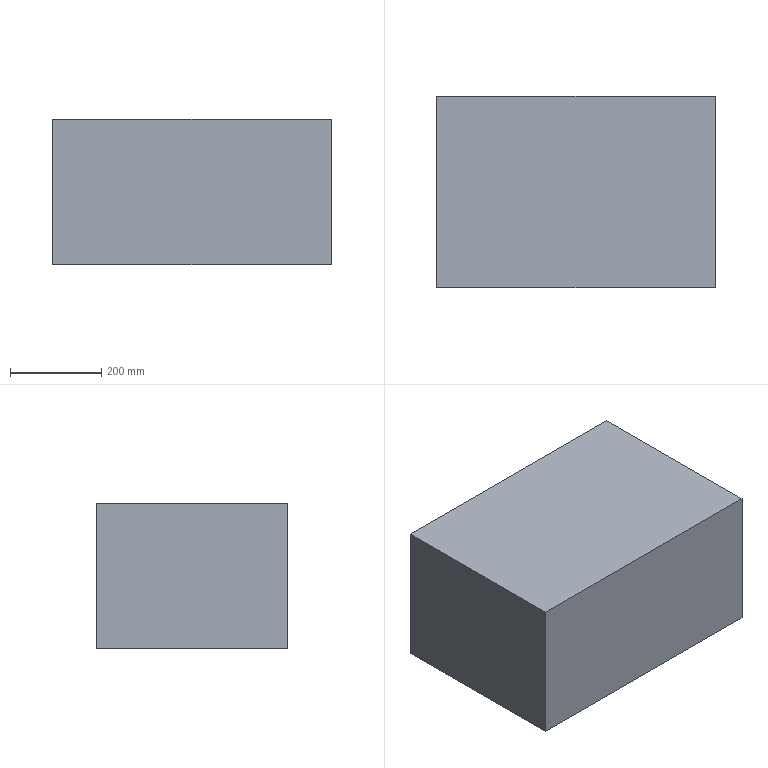Part | SolidWorks | features BaseBody 1 | 1 solid | 11 faces | box 610 x 420 x 320 mm | volume 8824000 mm3 | plane 11
STEP:
#1=CARTESIAN_POINT('',(295.,-200.,-10.));
#2=VERTEX_POINT('',#1);
#3=CARTESIAN_POINT('',(295.,200.,-10.));
#4=VERTEX_POINT('',#3);
#5=CARTESIAN_POINT('',(295.,0.,-10.));
#6=DIRECTION('',(0.,1.,0.));
#7=VECTOR('',#6,1000.);
#8=LINE('',#5,#7);
#9=EDGE_CURVE('',#2,#4,#8,.T.);
#10=ORIENTED_EDGE('',*,*,#9,.F.);
#11=CARTESIAN_POINT('',(-295.,-200.,-10.));
#12=VERTEX_POINT('',#11);
#13=CARTESIAN_POINT('',(0.,-200.,-10.));
#14=DIRECTION('',(1.,0.,0.));
#15=VECTOR('',#14,1000.);
#16=LINE('',#13,#15);
#17=EDGE_CURVE('',#12,#2,#16,.T.);
#18=ORIENTED_EDGE('',*,*,#17,.F.);
#19=CARTESIAN_POINT('',(-295.,200.,-10.));
#20=VERTEX_POINT('',#19);
#21=CARTESIAN_POINT('',(-295.,0.,-10.));
#22=DIRECTION('',(0.,-1.,0.));
#23=VECTOR('',#22,1000.);
#24=LINE('',#21,#23);
#25=EDGE_CURVE('',#20,#12,#24,.T.);
#26=ORIENTED_EDGE('',*,*,#25,.F.);
#27=CARTESIAN_POINT('',(0.,200.,-10.));
#28=DIRECTION('',(-1.,0.,0.));
#29=VECTOR('',#28,1000.);
#30=LINE('',#27,#29);
#31=EDGE_CURVE('',#4,#20,#30,.T.);
#32=ORIENTED_EDGE('',*,*,#31,.F.);
#33=EDGE_LOOP('',(#10,#18,#26,#32));
#34=FACE_OUTER_BOUND('',#33,.T.);
#35=CARTESIAN_POINT('',(0.,0.,-10.));
#36=DIRECTION('',(0.,0.,1.));
#37=DIRECTION('',(1.,0.,0.));
#38=AXIS2_PLACEMENT_3D('',#35,#36,#37);
#39=PLANE('',#38);
#40=ADVANCED_FACE('',(#34),#39,.F.);
#41=ORIENTED_EDGE('',*,*,#31,.T.);
#42=CARTESIAN_POINT('',(-295.,200.,-320.));
#43=VERTEX_POINT('',#42);
#44=CARTESIAN_POINT('',(-295.,200.,-320.));
#45=DIRECTION('',(0.,0.,1.));
#46=VECTOR('',#45,1000.);
#47=LINE('',#44,#46);
#48=EDGE_CURVE('',#43,#20,#47,.T.);
#49=ORIENTED_EDGE('',*,*,#48,.F.);
#50=CARTESIAN_POINT('',(295.,200.,-320.));
#51=VERTEX_POINT('',#50);
#52=CARTESIAN_POINT('',(0.,200.,-320.));
#53=DIRECTION('',(-1.,0.,0.));
#54=VECTOR('',#53,1000.);
#55=LINE('',#52,#54);
#56=EDGE_CURVE('',#51,#43,#55,.T.);
#57=ORIENTED_EDGE('',*,*,#56,.F.);
#58=CARTESIAN_POINT('',(295.,200.,-320.));
#59=DIRECTION('',(0.,0.,1.));
#60=VECTOR('',#59,1000.);
#61=LINE('',#58,#60);
#62=EDGE_CURVE('',#51,#4,#61,.T.);
#63=ORIENTED_EDGE('',*,*,#62,.T.);
#64=EDGE_LOOP('',(#41,#49,#57,#63));
#65=FACE_OUTER_BOUND('',#64,.T.);
#66=CARTESIAN_POINT('',(-305.,200.,-320.));
#67=DIRECTION('',(0.,1.,0.));
#68=DIRECTION('',(1.,0.,0.));
#69=AXIS2_PLACEMENT_3D('',#66,#67,#68);
#70=PLANE('',#69);
#71=ADVANCED_FACE('',(#65),#70,.F.);
#72=ORIENTED_EDGE('',*,*,#25,.T.);
#73=CARTESIAN_POINT('',(-295.,-200.,-320.));
#74=VERTEX_POINT('',#73);
#75=CARTESIAN_POINT('',(-295.,-200.,-320.));
#76=DIRECTION('',(0.,0.,1.));
#77=VECTOR('',#76,1000.);
#78=LINE('',#75,#77);
#79=EDGE_CURVE('',#74,#12,#78,.T.);
#80=ORIENTED_EDGE('',*,*,#79,.F.);
#81=CARTESIAN_POINT('',(-295.,0.,-320.));
#82=DIRECTION('',(0.,-1.,0.));
#83=VECTOR('',#82,1000.);
#84=LINE('',#81,#83);
#85=EDGE_CURVE('',#43,#74,#84,.T.);
#86=ORIENTED_EDGE('',*,*,#85,.F.);
#87=ORIENTED_EDGE('',*,*,#48,.T.);
#88=EDGE_LOOP('',(#72,#80,#86,#87));
#89=FACE_OUTER_BOUND('',#88,.T.);
#90=CARTESIAN_POINT('',(-295.,210.,-320.));
#91=DIRECTION('',(-1.,0.,0.));
#92=DIRECTION('',(0.,1.,0.));
#93=AXIS2_PLACEMENT_3D('',#90,#91,#92);
#94=PLANE('',#93);
#95=ADVANCED_FACE('',(#89),#94,.F.);
#96=ORIENTED_EDGE('',*,*,#17,.T.);
#97=CARTESIAN_POINT('',(295.,-200.,-320.));
#98=VERTEX_POINT('',#97);
#99=CARTESIAN_POINT('',(295.,-200.,-320.));
#100=DIRECTION('',(0.,0.,1.));
#101=VECTOR('',#100,1000.);
#102=LINE('',#99,#101);
#103=EDGE_CURVE('',#98,#2,#102,.T.);
#104=ORIENTED_EDGE('',*,*,#103,.F.);
#105=CARTESIAN_POINT('',(0.,-200.,-320.));
#106=DIRECTION('',(1.,0.,0.));
#107=VECTOR('',#106,1000.);
#108=LINE('',#105,#107);
#109=EDGE_CURVE('',#74,#98,#108,.T.);
#110=ORIENTED_EDGE('',*,*,#109,.F.);
#111=ORIENTED_EDGE('',*,*,#79,.T.);
#112=EDGE_LOOP('',(#96,#104,#110,#111));
#113=FACE_OUTER_BOUND('',#112,.T.);
#114=CARTESIAN_POINT('',(-305.,-200.,-320.));
#115=DIRECTION('',(0.,-1.,0.));
#116=DIRECTION('',(0.,0.,-1.));
#117=AXIS2_PLACEMENT_3D('',#114,#115,#116);
#118=PLANE('',#117);
#119=ADVANCED_FACE('',(#113),#118,.F.);
#120=ORIENTED_EDGE('',*,*,#9,.T.);
#121=ORIENTED_EDGE('',*,*,#62,.F.);
#122=CARTESIAN_POINT('',(295.,0.,-320.));
#123=DIRECTION('',(0.,1.,0.));
#124=VECTOR('',#123,1000.);
#125=LINE('',#122,#124);
#126=EDGE_CURVE('',#98,#51,#125,.T.);
#127=ORIENTED_EDGE('',*,*,#126,.F.);
#128=ORIENTED_EDGE('',*,*,#103,.T.);
#129=EDGE_LOOP('',(#120,#121,#127,#128));
#130=FACE_OUTER_BOUND('',#129,.T.);
#131=CARTESIAN_POINT('',(295.,210.,-320.));
#132=DIRECTION('',(1.,0.,0.));
#133=DIRECTION('',(0.,1.,0.));
#134=AXIS2_PLACEMENT_3D('',#131,#132,#133);
#135=PLANE('',#134);
#136=ADVANCED_FACE('',(#130),#135,.F.);
#137=CARTESIAN_POINT('',(305.,-210.,0.));
#138=VERTEX_POINT('',#137);
#139=CARTESIAN_POINT('',(305.,210.,0.));
#140=VERTEX_POINT('',#139);
#141=CARTESIAN_POINT('',(305.,210.,0.));
#142=DIRECTION('',(0.,1.,0.));
#143=VECTOR('',#142,1000.);
#144=LINE('',#141,#143);
#145=EDGE_CURVE('',#138,#140,#144,.T.);
#146=ORIENTED_EDGE('',*,*,#145,.T.);
#147=CARTESIAN_POINT('',(-305.,210.,0.));
#148=VERTEX_POINT('',#147);
#149=CARTESIAN_POINT('',(-305.,210.,0.));
#150=DIRECTION('',(-1.,0.,0.));
#151=VECTOR('',#150,1000.);
#152=LINE('',#149,#151);
#153=EDGE_CURVE('',#140,#148,#152,.T.);
#154=ORIENTED_EDGE('',*,*,#153,.T.);
#155=CARTESIAN_POINT('',(-305.,-210.,0.));
#156=VERTEX_POINT('',#155);
#157=CARTESIAN_POINT('',(-305.,210.,0.));
#158=DIRECTION('',(0.,-1.,0.));
#159=VECTOR('',#158,1000.);
#160=LINE('',#157,#159);
#161=EDGE_CURVE('',#148,#156,#160,.T.);
#162=ORIENTED_EDGE('',*,*,#161,.T.);
#163=CARTESIAN_POINT('',(-305.,-210.,0.));
#164=DIRECTION('',(1.,0.,0.));
#165=VECTOR('',#164,1000.);
#166=LINE('',#163,#165);
#167=EDGE_CURVE('',#156,#138,#166,.T.);
#168=ORIENTED_EDGE('',*,*,#167,.T.);
#169=EDGE_LOOP('',(#146,#154,#162,#168));
#170=FACE_OUTER_BOUND('',#169,.T.);
#171=CARTESIAN_POINT('',(0.,0.,0.));
#172=DIRECTION('',(0.,0.,1.));
#173=DIRECTION('',(1.,0.,0.));
#174=AXIS2_PLACEMENT_3D('',#171,#172,#173);
#175=PLANE('',#174);
#176=ADVANCED_FACE('',(#170),#175,.T.);
#177=ORIENTED_EDGE('',*,*,#109,.T.);
#178=ORIENTED_EDGE('',*,*,#126,.T.);
#179=ORIENTED_EDGE('',*,*,#56,.T.);
#180=ORIENTED_EDGE('',*,*,#85,.T.);
#181=EDGE_LOOP('',(#177,#178,#179,#180));
#182=FACE_BOUND('',#181,.T.);
#183=CARTESIAN_POINT('',(305.,-210.,-320.));
#184=VERTEX_POINT('',#183);
#185=CARTESIAN_POINT('',(305.,210.,-320.));
#186=VERTEX_POINT('',#185);
#187=CARTESIAN_POINT('',(305.,210.,-320.));
#188=DIRECTION('',(0.,1.,0.));
#189=VECTOR('',#188,1000.);
#190=LINE('',#187,#189);
#191=EDGE_CURVE('',#184,#186,#190,.T.);
#192=ORIENTED_EDGE('',*,*,#191,.F.);
#193=CARTESIAN_POINT('',(-305.,-210.,-320.));
#194=VERTEX_POINT('',#193);
#195=CARTESIAN_POINT('',(-305.,-210.,-320.));
#196=DIRECTION('',(1.,0.,0.));
#197=VECTOR('',#196,1000.);
#198=LINE('',#195,#197);
#199=EDGE_CURVE('',#194,#184,#198,.T.);
#200=ORIENTED_EDGE('',*,*,#199,.F.);
#201=CARTESIAN_POINT('',(-305.,210.,-320.));
#202=VERTEX_POINT('',#201);
#203=CARTESIAN_POINT('',(-305.,210.,-320.));
#204=DIRECTION('',(0.,-1.,0.));
#205=VECTOR('',#204,1000.);
#206=LINE('',#203,#205);
#207=EDGE_CURVE('',#202,#194,#206,.T.);
#208=ORIENTED_EDGE('',*,*,#207,.F.);
#209=CARTESIAN_POINT('',(-305.,210.,-320.));
#210=DIRECTION('',(-1.,0.,0.));
#211=VECTOR('',#210,1000.);
#212=LINE('',#209,#211);
#213=EDGE_CURVE('',#186,#202,#212,.T.);
#214=ORIENTED_EDGE('',*,*,#213,.F.);
#215=EDGE_LOOP('',(#192,#200,#208,#214));
#216=FACE_OUTER_BOUND('',#215,.T.);
#217=CARTESIAN_POINT('',(0.,0.,-320.));
#218=DIRECTION('',(0.,0.,1.));
#219=DIRECTION('',(1.,0.,0.));
#220=AXIS2_PLACEMENT_3D('',#217,#218,#219);
#221=PLANE('',#220);
#222=ADVANCED_FACE('',(#182,#216),#221,.F.);
#223=ORIENTED_EDGE('',*,*,#153,.F.);
#224=CARTESIAN_POINT('',(305.,210.,-320.));
#225=DIRECTION('',(0.,0.,1.));
#226=VECTOR('',#225,1000.);
#227=LINE('',#224,#226);
#228=EDGE_CURVE('',#186,#140,#227,.T.);
#229=ORIENTED_EDGE('',*,*,#228,.F.);
#230=ORIENTED_EDGE('',*,*,#213,.T.);
#231=CARTESIAN_POINT('',(-305.,210.,-320.));
#232=DIRECTION('',(0.,0.,1.));
#233=VECTOR('',#232,1000.);
#234=LINE('',#231,#233);
#235=EDGE_CURVE('',#202,#148,#234,.T.);
#236=ORIENTED_EDGE('',*,*,#235,.T.);
#237=EDGE_LOOP('',(#223,#229,#230,#236));
#238=FACE_OUTER_BOUND('',#237,.T.);
#239=CARTESIAN_POINT('',(-305.,210.,-320.));
#240=DIRECTION('',(0.,1.,0.));
#241=DIRECTION('',(1.,0.,0.));
#242=AXIS2_PLACEMENT_3D('',#239,#240,#241);
#243=PLANE('',#242);
#244=ADVANCED_FACE('',(#238),#243,.T.);
#245=ORIENTED_EDGE('',*,*,#161,.F.);
#246=ORIENTED_EDGE('',*,*,#235,.F.);
#247=ORIENTED_EDGE('',*,*,#207,.T.);
#248=CARTESIAN_POINT('',(-305.,-210.,-320.));
#249=DIRECTION('',(0.,0.,1.));
#250=VECTOR('',#249,1000.);
#251=LINE('',#248,#250);
#252=EDGE_CURVE('',#194,#156,#251,.T.);
#253=ORIENTED_EDGE('',*,*,#252,.T.);
#254=EDGE_LOOP('',(#245,#246,#247,#253));
#255=FACE_OUTER_BOUND('',#254,.T.);
#256=CARTESIAN_POINT('',(-305.,210.,-320.));
#257=DIRECTION('',(-1.,0.,0.));
#258=DIRECTION('',(0.,1.,0.));
#259=AXIS2_PLACEMENT_3D('',#256,#257,#258);
#260=PLANE('',#259);
#261=ADVANCED_FACE('',(#255),#260,.T.);
#262=ORIENTED_EDGE('',*,*,#167,.F.);
#263=ORIENTED_EDGE('',*,*,#252,.F.);
#264=ORIENTED_EDGE('',*,*,#199,.T.);
#265=CARTESIAN_POINT('',(305.,-210.,-320.));
#266=DIRECTION('',(0.,0.,1.));
#267=VECTOR('',#266,1000.);
#268=LINE('',#265,#267);
#269=EDGE_CURVE('',#184,#138,#268,.T.);
#270=ORIENTED_EDGE('',*,*,#269,.T.);
#271=EDGE_LOOP('',(#262,#263,#264,#270));
#272=FACE_OUTER_BOUND('',#271,.T.);
#273=CARTESIAN_POINT('',(-305.,-210.,-320.));
#274=DIRECTION('',(0.,-1.,0.));
#275=DIRECTION('',(0.,0.,-1.));
#276=AXIS2_PLACEMENT_3D('',#273,#274,#275);
#277=PLANE('',#276);
#278=ADVANCED_FACE('',(#272),#277,.T.);
#279=ORIENTED_EDGE('',*,*,#145,.F.);
#280=ORIENTED_EDGE('',*,*,#269,.F.);
#281=ORIENTED_EDGE('',*,*,#191,.T.);
#282=ORIENTED_EDGE('',*,*,#228,.T.);
#283=EDGE_LOOP('',(#279,#280,#281,#282));
#284=FACE_OUTER_BOUND('',#283,.T.);
#285=CARTESIAN_POINT('',(305.,210.,-320.));
#286=DIRECTION('',(1.,0.,0.));
#287=DIRECTION('',(0.,1.,0.));
#288=AXIS2_PLACEMENT_3D('',#285,#286,#287);
#289=PLANE('',#288);
#290=ADVANCED_FACE('',(#284),#289,.T.);
#291=CLOSED_SHELL('',(#40,#71,#95,#119,#136,#176,#222,#244,#261,#278,#290));
#292=MANIFOLD_SOLID_BREP('',#291);
#293=CARTESIAN_POINT('',(0.,0.,0.));
#294=DIRECTION('',(0.,0.,1.));
#295=DIRECTION('',(1.,0.,0.));
#296=AXIS2_PLACEMENT_3D('',#293,#294,#295);
#297=(LENGTH_UNIT()NAMED_UNIT(*)SI_UNIT(.MILLI.,.METRE.));
#298=UNCERTAINTY_MEASURE_WITH_UNIT(LENGTH_MEASURE(0.00001),#297,'','');
#299=(NAMED_UNIT(*)PLANE_ANGLE_UNIT()SI_UNIT($,.RADIAN.));
#300=(NAMED_UNIT(*)SI_UNIT($,.STERADIAN.)SOLID_ANGLE_UNIT());
#301=(GEOMETRIC_REPRESENTATION_CONTEXT(3)GLOBAL_UNCERTAINTY_ASSIGNED_CONTEXT((#298))GLOBAL_UNIT_ASSIGNED_CONTEXT((#297,#299,#300))REPRESENTATION_CONTEXT('',''));
#302=ADVANCED_BREP_SHAPE_REPRESENTATION('',(#292,#296),#301);